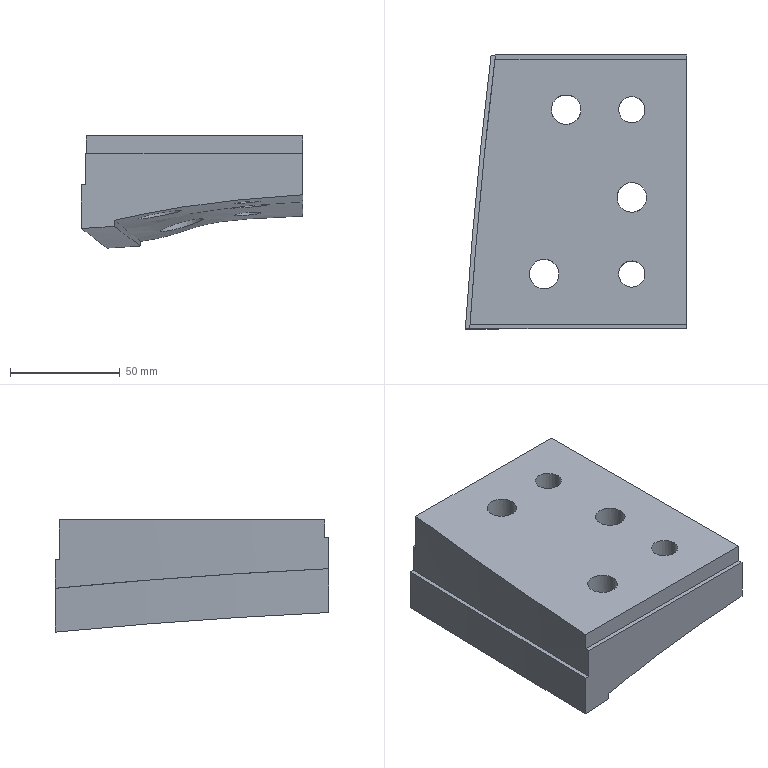Part | NX | features solid 2 | 1 solid | 25 faces | box 100.952 x 125 x 51.2 mm | volume 397040 mm3 | plane 10 | cylinder 8 | spline 7 | commonest cylinder face diameters 13.5 x3 20 x3 12 x2
STEP:
#1=CARTESIAN_POINT('',(-489.032,184.382,-45.));
#2=VERTEX_POINT('',#1);
#3=CARTESIAN_POINT('',(-490.817,179.819,-44.656));
#4=CARTESIAN_POINT('',(-488.384,184.323,-44.95));
#5=CARTESIAN_POINT('',(-489.838,189.179,-45.548));
#6=CARTESIAN_POINT('',(-494.281,191.609,-46.129));
#7=CARTESIAN_POINT('',(-499.185,190.178,-46.439));
#8=CARTESIAN_POINT('',(-501.615,185.671,-46.201));
#9=CARTESIAN_POINT('',(-500.164,180.829,-45.55));
#10=CARTESIAN_POINT('',(-495.732,178.391,-44.896));
#11=CARTESIAN_POINT('',(-490.817,179.819,-44.656));
#12=CARTESIAN_POINT('',(-488.384,184.323,-44.95));
#13=CARTESIAN_POINT('',(-489.838,189.179,-45.548));
#14=B_SPLINE_CURVE_WITH_KNOTS('',3,(#3,#4,#5,#6,#7,#8,#9,#10,#11,#12,#13),.UNSPECIFIED.,.T.,.F.,(1,1,1,1,1,1,1,1,1,1,1,1,1,1,1),(-0.01413,-0.009419,-0.00471,0.,0.00471,0.009419,0.01413,0.01884,0.02355,0.02826,0.03297,0.03768,0.04239,0.0471,0.05181),.UNSPECIFIED.);
#15=EDGE_CURVE('',#2,#2,#14,.T.);
#16=ORIENTED_EDGE('',*,*,#15,.T.);
#17=EDGE_LOOP('',(#16));
#18=FACE_BOUND('',#17,.T.);
#19=CARTESIAN_POINT('',(-485.058,146.073,-41.181));
#20=VERTEX_POINT('',#19);
#21=CARTESIAN_POINT('',(-488.05,153.62,-41.932));
#22=CARTESIAN_POINT('',(-483.979,146.199,-41.004));
#23=CARTESIAN_POINT('',(-486.381,138.023,-41.137));
#24=CARTESIAN_POINT('',(-492.586,134.671,-41.575));
#25=CARTESIAN_POINT('',(-497.883,135.157,-42.166));
#26=CARTESIAN_POINT('',(-501.42,136.996,-42.631));
#27=CARTESIAN_POINT('',(-504.,140.069,-42.843));
#28=CARTESIAN_POINT('',(-505.202,143.899,-42.744));
#29=CARTESIAN_POINT('',(-504.844,147.89,-42.805));
#30=CARTESIAN_POINT('',(-502.374,152.636,-42.99));
#31=CARTESIAN_POINT('',(-496.153,156.023,-42.778));
#32=CARTESIAN_POINT('',(-488.05,153.62,-41.932));
#33=CARTESIAN_POINT('',(-483.979,146.199,-41.004));
#34=CARTESIAN_POINT('',(-486.381,138.023,-41.137));
#35=B_SPLINE_CURVE_WITH_KNOTS('',3,(#21,#22,#23,#24,#25,#26,#27,#28,#29,#30,#31,#32,#33,#34),.UNSPECIFIED.,.T.,.F.,(1,1,1,1,1,1,1,1,1,1,1,1,1,1,1,1,1,1),(-0.0235,-0.01567,-0.007835,0.,0.007835,0.01567,0.01959,0.0235,0.02742,0.03134,0.03526,0.03917,0.04701,0.05484,0.06268,0.07051,0.07835,0.08226),.UNSPECIFIED.);
#36=EDGE_CURVE('',#20,#20,#35,.T.);
#37=ORIENTED_EDGE('',*,*,#36,.F.);
#38=EDGE_LOOP('',(#37));
#39=FACE_BOUND('',#38,.T.);
#40=CARTESIAN_POINT('',(-489.032,109.384,-39.583));
#41=VERTEX_POINT('',#40);
#42=CARTESIAN_POINT('',(-490.822,104.819,-39.486));
#43=CARTESIAN_POINT('',(-488.38,109.321,-39.523));
#44=CARTESIAN_POINT('',(-489.848,114.196,-39.92));
#45=CARTESIAN_POINT('',(-494.297,116.607,-40.474));
#46=CARTESIAN_POINT('',(-499.179,115.178,-40.9));
#47=CARTESIAN_POINT('',(-501.618,110.678,-40.908));
#48=CARTESIAN_POINT('',(-500.157,105.813,-40.46));
#49=CARTESIAN_POINT('',(-495.712,103.393,-39.862));
#50=CARTESIAN_POINT('',(-490.822,104.819,-39.486));
#51=CARTESIAN_POINT('',(-488.38,109.321,-39.523));
#52=CARTESIAN_POINT('',(-489.848,114.196,-39.92));
#53=B_SPLINE_CURVE_WITH_KNOTS('',3,(#42,#43,#44,#45,#46,#47,#48,#49,#50,#51,#52),.UNSPECIFIED.,.T.,.F.,(1,1,1,1,1,1,1,1,1,1,1,1,1,1,1),(-0.01411,-0.009409,-0.004704,0.,0.004704,0.009409,0.01411,0.01882,0.02352,0.02823,0.03293,0.03763,0.04234,0.04704,0.05175),.UNSPECIFIED.);
#54=EDGE_CURVE('',#41,#41,#53,.T.);
#55=ORIENTED_EDGE('',*,*,#54,.T.);
#56=EDGE_LOOP('',(#55));
#57=FACE_BOUND('',#56,.T.);
#58=CARTESIAN_POINT('',(-470.,85.,-36.878));
#59=VERTEX_POINT('',#58);
#60=CARTESIAN_POINT('',(-470.,210.,-46.611));
#61=VERTEX_POINT('',#60);
#62=CARTESIAN_POINT('',(-470.,85.,-36.878));
#63=CARTESIAN_POINT('',(-470.,90.22,-37.142));
#64=CARTESIAN_POINT('',(-470.,100.66,-37.689));
#65=CARTESIAN_POINT('',(-470.,113.71,-38.361));
#66=CARTESIAN_POINT('',(-470.,124.15,-38.933));
#67=CARTESIAN_POINT('',(-470.,131.966,-39.52));
#68=CARTESIAN_POINT('',(-470.,139.786,-40.056));
#69=CARTESIAN_POINT('',(-470.,150.223,-40.671));
#70=CARTESIAN_POINT('',(-470.,160.627,-41.624));
#71=CARTESIAN_POINT('',(-470.,171.035,-42.538));
#72=CARTESIAN_POINT('',(-470.,178.828,-43.35));
#73=CARTESIAN_POINT('',(-470.,186.628,-44.098));
#74=CARTESIAN_POINT('',(-470.,194.439,-44.73));
#75=CARTESIAN_POINT('',(-470.,202.242,-45.44));
#76=CARTESIAN_POINT('',(-470.,207.414,-46.217));
#77=CARTESIAN_POINT('',(-470.,210.,-46.611));
#78=B_SPLINE_CURVE_WITH_KNOTS('',3,(#62,#63,#64,#65,#66,#67,#68,#69,#70,#71,#72,#73,#74,#75,#76,#77),.UNSPECIFIED.,.F.,.F.,(4,1,1,1,1,1,1,1,1,1,1,1,1,4),(0.,0.01568,0.03136,0.0392,0.04704,0.05488,0.06272,0.07841,0.08625,0.09409,0.1019,0.1098,0.1176,0.1254),.UNSPECIFIED.);
#79=EDGE_CURVE('',#59,#61,#78,.T.);
#80=ORIENTED_EDGE('',*,*,#79,.F.);
#81=CARTESIAN_POINT('',(-555.921,85.,-48.486));
#82=VERTEX_POINT('',#81);
#83=CARTESIAN_POINT('',(-470.,85.,-36.878));
#84=CARTESIAN_POINT('',(-477.221,85.,-37.317));
#85=CARTESIAN_POINT('',(-491.647,85.,-38.355));
#86=CARTESIAN_POINT('',(-513.236,85.,-40.649));
#87=CARTESIAN_POINT('',(-531.108,85.,-43.363));
#88=CARTESIAN_POINT('',(-545.301,85.,-46.198));
#89=CARTESIAN_POINT('',(-552.373,85.,-47.779));
#90=CARTESIAN_POINT('',(-555.921,85.,-48.486));
#91=B_SPLINE_CURVE_WITH_KNOTS('',3,(#83,#84,#85,#86,#87,#88,#89,#90),.UNSPECIFIED.,.F.,.F.,(4,1,1,1,1,4),(0.,0.0217,0.04339,0.06509,0.07594,0.08679),.UNSPECIFIED.);
#92=EDGE_CURVE('',#59,#82,#91,.T.);
#93=ORIENTED_EDGE('',*,*,#92,.T.);
#94=CARTESIAN_POINT('',(-544.144,210.,-58.181));
#95=VERTEX_POINT('',#94);
#96=CARTESIAN_POINT('',(-555.921,85.,-48.486));
#97=CARTESIAN_POINT('',(-555.618,90.231,-48.778));
#98=CARTESIAN_POINT('',(-554.9,100.695,-49.199));
#99=CARTESIAN_POINT('',(-553.869,113.757,-49.868));
#100=CARTESIAN_POINT('',(-553.001,124.186,-50.711));
#101=CARTESIAN_POINT('',(-552.323,132.016,-51.197));
#102=CARTESIAN_POINT('',(-551.623,139.823,-51.95));
#103=CARTESIAN_POINT('',(-550.898,147.619,-52.805));
#104=CARTESIAN_POINT('',(-550.144,155.441,-53.298));
#105=CARTESIAN_POINT('',(-549.364,163.258,-53.831));
#106=CARTESIAN_POINT('',(-548.558,171.067,-54.429));
#107=CARTESIAN_POINT('',(-547.449,181.481,-55.148));
#108=CARTESIAN_POINT('',(-546.289,191.874,-56.065));
#109=CARTESIAN_POINT('',(-545.078,202.255,-57.078));
#110=CARTESIAN_POINT('',(-544.458,207.419,-57.811));
#111=CARTESIAN_POINT('',(-544.144,210.,-58.181));
#112=B_SPLINE_CURVE_WITH_KNOTS('',3,(#96,#97,#98,#99,#100,#101,#102,#103,#104,#105,#106,#107,#108,#109,#110,#111),.UNSPECIFIED.,.F.,.F.,(4,1,1,1,1,1,1,1,1,1,1,1,1,4),(0.,0.01574,0.03149,0.03936,0.04723,0.0551,0.06297,0.07084,0.07872,0.08659,0.09446,0.1102,0.1181,0.1259),.UNSPECIFIED.);
#113=EDGE_CURVE('',#82,#95,#112,.T.);
#114=ORIENTED_EDGE('',*,*,#113,.T.);
#115=CARTESIAN_POINT('',(-470.,210.,-46.611));
#116=CARTESIAN_POINT('',(-473.142,210.,-46.734));
#117=CARTESIAN_POINT('',(-479.425,210.,-46.986));
#118=CARTESIAN_POINT('',(-488.844,210.,-47.464));
#119=CARTESIAN_POINT('',(-498.259,210.,-48.122));
#120=CARTESIAN_POINT('',(-507.638,210.,-49.048));
#121=CARTESIAN_POINT('',(-516.834,210.,-50.901));
#122=CARTESIAN_POINT('',(-525.787,210.,-54.007));
#123=CARTESIAN_POINT('',(-534.818,210.,-56.749));
#124=CARTESIAN_POINT('',(-541.02,210.,-57.77));
#125=CARTESIAN_POINT('',(-544.144,210.,-58.181));
#126=B_SPLINE_CURVE_WITH_KNOTS('',3,(#115,#116,#117,#118,#119,#120,#121,#122,#123,#124,#125),.UNSPECIFIED.,.F.,.F.,(4,1,1,1,1,1,1,1,4),(0.01237,0.0218,0.03123,0.04067,0.0501,0.05953,0.06896,0.07839,0.08783),.UNSPECIFIED.);
#127=EDGE_CURVE('',#61,#95,#126,.T.);
#128=ORIENTED_EDGE('',*,*,#127,.F.);
#129=EDGE_LOOP('',(#80,#93,#114,#128));
#130=FACE_BOUND('',#129,.T.);
#131=CARTESIAN_POINT('',(-525.061,111.107,-44.092));
#132=VERTEX_POINT('',#131);
#133=CARTESIAN_POINT('',(-528.118,118.659,-45.091));
#134=CARTESIAN_POINT('',(-523.966,111.248,-43.923));
#135=CARTESIAN_POINT('',(-526.389,102.987,-43.772));
#136=CARTESIAN_POINT('',(-533.894,98.99,-44.809));
#137=CARTESIAN_POINT('',(-541.907,101.367,-46.521));
#138=CARTESIAN_POINT('',(-546.025,108.74,-47.878));
#139=CARTESIAN_POINT('',(-543.623,116.999,-48.006));
#140=CARTESIAN_POINT('',(-536.127,121.004,-46.796));
#141=CARTESIAN_POINT('',(-528.118,118.659,-45.091));
#142=CARTESIAN_POINT('',(-523.966,111.248,-43.923));
#143=CARTESIAN_POINT('',(-526.389,102.987,-43.772));
#144=B_SPLINE_CURVE_WITH_KNOTS('',3,(#133,#134,#135,#136,#137,#138,#139,#140,#141,#142,#143),.UNSPECIFIED.,.T.,.F.,(1,1,1,1,1,1,1,1,1,1,1,1,1,1,1),(-0.02369,-0.01579,-0.007895,0.,0.007895,0.01579,0.02369,0.03158,0.03948,0.04737,0.05527,0.06316,0.07106,0.07895,0.08685),.UNSPECIFIED.);
#145=EDGE_CURVE('',#132,#132,#144,.T.);
#146=ORIENTED_EDGE('',*,*,#145,.F.);
#147=EDGE_LOOP('',(#146));
#148=FACE_BOUND('',#147,.T.);
#149=CARTESIAN_POINT('',(-515.067,186.16,-48.081));
#150=VERTEX_POINT('',#149);
#151=CARTESIAN_POINT('',(-516.071,190.051,-48.693));
#152=CARTESIAN_POINT('',(-514.364,184.908,-47.814));
#153=CARTESIAN_POINT('',(-515.981,179.356,-47.499));
#154=CARTESIAN_POINT('',(-520.205,175.926,-48.09));
#155=CARTESIAN_POINT('',(-525.3,174.415,-49.332));
#156=CARTESIAN_POINT('',(-531.817,176.329,-51.579));
#157=CARTESIAN_POINT('',(-536.034,183.652,-53.385));
#158=CARTESIAN_POINT('',(-534.032,190.627,-53.73));
#159=CARTESIAN_POINT('',(-529.818,194.06,-53.026));
#160=CARTESIAN_POINT('',(-524.727,195.588,-51.756));
#161=CARTESIAN_POINT('',(-519.514,194.052,-49.991));
#162=CARTESIAN_POINT('',(-516.071,190.051,-48.693));
#163=CARTESIAN_POINT('',(-514.364,184.908,-47.814));
#164=CARTESIAN_POINT('',(-515.981,179.356,-47.499));
#165=B_SPLINE_CURVE_WITH_KNOTS('',3,(#151,#152,#153,#154,#155,#156,#157,#158,#159,#160,#161,#162,#163,#164),.UNSPECIFIED.,.T.,.F.,(1,1,1,1,1,1,1,1,1,1,1,1,1,1,1,1,1,1),(-0.01598,-0.00799,-0.003995,0.,0.00799,0.01198,0.01598,0.02397,0.03196,0.03995,0.04394,0.04794,0.05593,0.05992,0.06392,0.07191,0.0759,0.0799),.UNSPECIFIED.);
#166=EDGE_CURVE('',#150,#150,#165,.T.);
#167=ORIENTED_EDGE('',*,*,#166,.F.);
#168=EDGE_LOOP('',(#167));
#169=FACE_BOUND('',#168,.T.);
#170=CARTESIAN_POINT('',(-460.236,210.,-46.224));
#171=CARTESIAN_POINT('',(-460.402,208.227,-46.015));
#172=CARTESIAN_POINT('',(-460.814,203.794,-45.453));
#173=CARTESIAN_POINT('',(-461.733,195.358,-44.345));
#174=CARTESIAN_POINT('',(-462.841,184.682,-43.676));
#175=CARTESIAN_POINT('',(-463.729,174.009,-42.571));
#176=CARTESIAN_POINT('',(-464.671,164.665,-41.767));
#177=CARTESIAN_POINT('',(-465.319,155.367,-40.993));
#178=CARTESIAN_POINT('',(-465.637,145.924,-40.241));
#179=CARTESIAN_POINT('',(-466.776,135.731,-39.584));
#180=CARTESIAN_POINT('',(-467.28,126.264,-38.89));
#181=CARTESIAN_POINT('',(-467.918,115.603,-38.325));
#182=CARTESIAN_POINT('',(-468.419,106.237,-37.886));
#183=CARTESIAN_POINT('',(-468.993,95.595,-37.354));
#184=CARTESIAN_POINT('',(-469.29,88.96,-37.034));
#185=CARTESIAN_POINT('',(-469.48,85.,-36.847));
#186=CARTESIAN_POINT('',(-460.832,210.,-46.249));
#187=CARTESIAN_POINT('',(-460.999,208.227,-46.037));
#188=CARTESIAN_POINT('',(-461.414,203.794,-45.469));
#189=CARTESIAN_POINT('',(-462.332,195.358,-44.372));
#190=CARTESIAN_POINT('',(-463.441,184.682,-43.699));
#191=CARTESIAN_POINT('',(-464.331,174.009,-42.593));
#192=CARTESIAN_POINT('',(-465.273,164.665,-41.788));
#193=CARTESIAN_POINT('',(-465.922,155.367,-41.015));
#194=CARTESIAN_POINT('',(-466.245,145.924,-40.257));
#195=CARTESIAN_POINT('',(-467.376,135.731,-39.626));
#196=CARTESIAN_POINT('',(-467.882,126.264,-38.927));
#197=CARTESIAN_POINT('',(-468.521,115.603,-38.363));
#198=CARTESIAN_POINT('',(-469.022,106.237,-37.923));
#199=CARTESIAN_POINT('',(-469.597,95.595,-37.391));
#200=CARTESIAN_POINT('',(-469.894,88.96,-37.072));
#201=CARTESIAN_POINT('',(-470.084,85.,-36.883));
#202=CARTESIAN_POINT('',(-473.295,210.,-46.76));
#203=CARTESIAN_POINT('',(-473.479,208.227,-46.49));
#204=CARTESIAN_POINT('',(-473.937,203.794,-45.772));
#205=CARTESIAN_POINT('',(-474.839,195.358,-44.949));
#206=CARTESIAN_POINT('',(-475.975,184.682,-44.202));
#207=CARTESIAN_POINT('',(-476.895,174.009,-43.072));
#208=CARTESIAN_POINT('',(-477.842,164.665,-42.233));
#209=CARTESIAN_POINT('',(-478.513,155.367,-41.491));
#210=CARTESIAN_POINT('',(-478.929,145.924,-40.6));
#211=CARTESIAN_POINT('',(-479.904,135.731,-40.535));
#212=CARTESIAN_POINT('',(-480.465,126.264,-39.711));
#213=CARTESIAN_POINT('',(-481.107,115.603,-39.168));
#214=CARTESIAN_POINT('',(-481.621,106.237,-38.712));
#215=CARTESIAN_POINT('',(-482.207,95.595,-38.169));
#216=CARTESIAN_POINT('',(-482.509,88.96,-37.871));
#217=CARTESIAN_POINT('',(-482.705,85.,-37.654));
#218=CARTESIAN_POINT('',(-491.74,210.,-47.323));
#219=CARTESIAN_POINT('',(-491.958,208.227,-46.857));
#220=CARTESIAN_POINT('',(-492.499,203.794,-45.664));
#221=CARTESIAN_POINT('',(-493.223,195.358,-46.413));
#222=CARTESIAN_POINT('',(-494.458,184.682,-45.146));
#223=CARTESIAN_POINT('',(-495.396,174.009,-44.159));
#224=CARTESIAN_POINT('',(-496.354,164.665,-43.256));
#225=CARTESIAN_POINT('',(-497.049,155.367,-42.572));
#226=CARTESIAN_POINT('',(-497.612,145.924,-41.455));
#227=CARTESIAN_POINT('',(-498.346,135.731,-42.296));
#228=CARTESIAN_POINT('',(-498.993,126.264,-41.259));
#229=CARTESIAN_POINT('',(-499.642,115.603,-40.736));
#230=CARTESIAN_POINT('',(-500.178,106.237,-40.249));
#231=CARTESIAN_POINT('',(-500.78,95.595,-39.695));
#232=CARTESIAN_POINT('',(-501.087,88.96,-39.432));
#233=CARTESIAN_POINT('',(-501.293,85.,-39.169));
#234=CARTESIAN_POINT('',(-515.308,210.,-49.876));
#235=CARTESIAN_POINT('',(-515.383,208.227,-50.08));
#236=CARTESIAN_POINT('',(-515.547,203.794,-50.668));
#237=CARTESIAN_POINT('',(-516.964,195.358,-48.656));
#238=CARTESIAN_POINT('',(-518.105,184.682,-47.911));
#239=CARTESIAN_POINT('',(-519.113,174.009,-46.903));
#240=CARTESIAN_POINT('',(-520.049,164.665,-46.195));
#241=CARTESIAN_POINT('',(-520.752,155.367,-45.521));
#242=CARTESIAN_POINT('',(-521.536,145.924,-44.162));
#243=CARTESIAN_POINT('',(-521.95,135.731,-45.834));
#244=CARTESIAN_POINT('',(-522.72,126.264,-44.564));
#245=CARTESIAN_POINT('',(-523.391,115.603,-44.003));
#246=CARTESIAN_POINT('',(-523.962,106.237,-43.458));
#247=CARTESIAN_POINT('',(-524.585,95.595,-42.914));
#248=CARTESIAN_POINT('',(-524.893,88.96,-42.673));
#249=CARTESIAN_POINT('',(-525.118,85.,-42.375));
#250=CARTESIAN_POINT('',(-530.676,210.,-56.049));
#251=CARTESIAN_POINT('',(-530.891,208.227,-55.766));
#252=CARTESIAN_POINT('',(-531.432,203.794,-55.039));
#253=CARTESIAN_POINT('',(-532.529,195.358,-54.442));
#254=CARTESIAN_POINT('',(-533.734,184.682,-53.359));
#255=CARTESIAN_POINT('',(-534.746,174.009,-52.593));
#256=CARTESIAN_POINT('',(-535.674,164.665,-51.937));
#257=CARTESIAN_POINT('',(-536.473,155.367,-51.094));
#258=CARTESIAN_POINT('',(-537.062,145.924,-50.979));
#259=CARTESIAN_POINT('',(-538.426,135.731,-47.973));
#260=CARTESIAN_POINT('',(-538.988,126.264,-47.837));
#261=CARTESIAN_POINT('',(-539.746,115.603,-46.909));
#262=CARTESIAN_POINT('',(-540.322,106.237,-46.4));
#263=CARTESIAN_POINT('',(-540.959,95.595,-45.863));
#264=CARTESIAN_POINT('',(-541.28,88.96,-45.6));
#265=CARTESIAN_POINT('',(-541.504,85.,-45.321));
#266=CARTESIAN_POINT('',(-540.959,210.,-57.8));
#267=CARTESIAN_POINT('',(-541.189,208.227,-57.529));
#268=CARTESIAN_POINT('',(-541.763,203.794,-56.829));
#269=CARTESIAN_POINT('',(-542.769,195.358,-56.095));
#270=CARTESIAN_POINT('',(-543.985,184.682,-55.045));
#271=CARTESIAN_POINT('',(-545.01,174.009,-54.312));
#272=CARTESIAN_POINT('',(-545.933,164.665,-53.616));
#273=CARTESIAN_POINT('',(-546.774,155.367,-52.906));
#274=CARTESIAN_POINT('',(-547.385,145.924,-52.438));
#275=CARTESIAN_POINT('',(-548.794,135.731,-50.689));
#276=CARTESIAN_POINT('',(-549.359,126.264,-50.207));
#277=CARTESIAN_POINT('',(-550.134,115.603,-49.305));
#278=CARTESIAN_POINT('',(-550.722,106.237,-48.739));
#279=CARTESIAN_POINT('',(-551.359,95.595,-48.242));
#280=CARTESIAN_POINT('',(-551.705,88.96,-47.933));
#281=CARTESIAN_POINT('',(-551.912,85.,-47.697));
#282=CARTESIAN_POINT('',(-545.458,210.,-58.347));
#283=CARTESIAN_POINT('',(-545.688,208.227,-58.102));
#284=CARTESIAN_POINT('',(-546.261,203.794,-57.465));
#285=CARTESIAN_POINT('',(-547.264,195.358,-56.552));
#286=CARTESIAN_POINT('',(-548.481,184.682,-55.532));
#287=CARTESIAN_POINT('',(-549.517,174.009,-54.789));
#288=CARTESIAN_POINT('',(-550.439,164.665,-54.063));
#289=CARTESIAN_POINT('',(-551.292,155.367,-53.425));
#290=CARTESIAN_POINT('',(-551.937,145.924,-52.754));
#291=CARTESIAN_POINT('',(-553.279,135.731,-51.737));
#292=CARTESIAN_POINT('',(-553.867,126.264,-51.07));
#293=CARTESIAN_POINT('',(-554.644,115.603,-50.203));
#294=CARTESIAN_POINT('',(-555.239,106.237,-49.615));
#295=CARTESIAN_POINT('',(-555.877,95.595,-49.132));
#296=CARTESIAN_POINT('',(-556.23,88.96,-48.813));
#297=CARTESIAN_POINT('',(-556.433,85.,-48.587));
#298=B_SPLINE_SURFACE_WITH_KNOTS('',3,3,((#170,#171,#172,#173,#174,#175,#176,#177,#178,#179,#180,#181,#182,#183,#184,#185),(#186,#187,#188,#189,#190,#191,#192,#193,#194,#195,#196,#197,#198,#199,#200,#201),(#202,#203,#204,#205,#206,#207,#208,#209,#210,#211,#212,#213,#214,#215,#216,#217),(#218,#219,#220,#221,#222,#223,#224,#225,#226,#227,#228,#229,#230,#231,#232,#233),(#234,#235,#236,#237,#238,#239,#240,#241,#242,#243,#244,#245,#246,#247,#248,#249),(#250,#251,#252,#253,#254,#255,#256,#257,#258,#259,#260,#261,#262,#263,#264,#265),(#266,#267,#268,#269,#270,#271,#272,#273,#274,#275,#276,#277,#278,#279,#280,#281),(#282,#283,#284,#285,#286,#287,#288,#289,#290,#291,#292,#293,#294,#295,#296,#297)),.UNSPECIFIED.,.F.,.F.,.F.,(4,1,1,1,1,4),(4,1,1,1,1,1,1,1,1,1,1,1,1,4),(0.9047,0.9062,0.9375,0.9531,0.9688,0.9807),(0.5208,0.5312,0.5469,0.5703,0.5938,0.6094,0.625,0.6484,0.6641,0.6875,0.7031,0.7266,0.7422,0.7653),.UNSPECIFIED.);
#299=ADVANCED_FACE('',(#18,#39,#57,#130,#148,#169),#298,.F.);
#300=CARTESIAN_POINT('',(-470.,210.,-28.));
#301=VERTEX_POINT('',#300);
#302=CARTESIAN_POINT('',(-470.,210.,-43.841));
#303=DIRECTION('',(0.,0.,1.));
#304=VECTOR('',#303,1000.);
#305=LINE('',#302,#304);
#306=EDGE_CURVE('',#301,#61,#305,.F.);
#307=ORIENTED_EDGE('',*,*,#306,.T.);
#308=ORIENTED_EDGE('',*,*,#127,.T.);
#309=CARTESIAN_POINT('',(-544.144,210.,-60.227));
#310=VERTEX_POINT('',#309);
#311=CARTESIAN_POINT('',(-544.144,210.,-63.127));
#312=DIRECTION('',(0.,0.,1.));
#313=VECTOR('',#312,1000.);
#314=LINE('',#311,#313);
#315=EDGE_CURVE('',#310,#95,#314,.T.);
#316=ORIENTED_EDGE('',*,*,#315,.F.);
#317=CARTESIAN_POINT('',(-559.253,210.,-61.2));
#318=VERTEX_POINT('',#317);
#319=CARTESIAN_POINT('',(-559.253,210.,-61.2));
#320=CARTESIAN_POINT('',(-554.217,210.,-60.868));
#321=CARTESIAN_POINT('',(-549.18,210.,-60.544));
#322=CARTESIAN_POINT('',(-544.144,210.,-60.227));
#323=B_SPLINE_CURVE_WITH_KNOTS('',3,(#319,#320,#321,#322),.UNSPECIFIED.,.F.,.F.,(4,4),(0.01195,0.02709),.UNSPECIFIED.);
#324=EDGE_CURVE('',#318,#310,#323,.T.);
#325=ORIENTED_EDGE('',*,*,#324,.F.);
#326=CARTESIAN_POINT('',(-559.253,210.,-41.2));
#327=VERTEX_POINT('',#326);
#328=CARTESIAN_POINT('',(-559.253,210.,-55.491));
#329=DIRECTION('',(0.,0.,1.));
#330=VECTOR('',#329,1000.);
#331=LINE('',#328,#330);
#332=EDGE_CURVE('',#327,#318,#331,.F.);
#333=ORIENTED_EDGE('',*,*,#332,.F.);
#334=CARTESIAN_POINT('',(-557.238,210.,-41.223));
#335=VERTEX_POINT('',#334);
#336=CARTESIAN_POINT('',(-557.238,210.,-41.223));
#337=CARTESIAN_POINT('',(-557.91,210.,-41.215));
#338=CARTESIAN_POINT('',(-558.581,210.,-41.208));
#339=CARTESIAN_POINT('',(-559.253,210.,-41.2));
#340=B_SPLINE_CURVE_WITH_KNOTS('',3,(#336,#337,#338,#339),.UNSPECIFIED.,.F.,.F.,(4,4),(0.,0.002015),.UNSPECIFIED.);
#341=EDGE_CURVE('',#335,#327,#340,.T.);
#342=ORIENTED_EDGE('',*,*,#341,.F.);
#343=CARTESIAN_POINT('',(-557.238,210.,-28.));
#344=VERTEX_POINT('',#343);
#345=CARTESIAN_POINT('',(-557.238,210.,-8.291));
#346=DIRECTION('',(0.,0.,1.));
#347=VECTOR('',#346,1000.);
#348=LINE('',#345,#347);
#349=EDGE_CURVE('',#344,#335,#348,.F.);
#350=ORIENTED_EDGE('',*,*,#349,.F.);
#351=CARTESIAN_POINT('',(-557.238,210.,-28.));
#352=DIRECTION('',(-1.,0.,0.));
#353=VECTOR('',#352,1000.);
#354=LINE('',#351,#353);
#355=EDGE_CURVE('',#344,#301,#354,.F.);
#356=ORIENTED_EDGE('',*,*,#355,.T.);
#357=EDGE_LOOP('',(#307,#308,#316,#325,#333,#342,#350,#356));
#358=FACE_BOUND('',#357,.T.);
#359=CARTESIAN_POINT('',(-130.,210.,-36.981));
#360=DIRECTION('',(0.,1.,0.));
#361=DIRECTION('',(0.,0.,1.));
#362=AXIS2_PLACEMENT_3D('',#359,#360,#361);
#363=PLANE('',#362);
#364=ADVANCED_FACE('',(#358),#363,.T.);
#365=CARTESIAN_POINT('',(-470.,208.,-10.));
#366=VERTEX_POINT('',#365);
#367=CARTESIAN_POINT('',(-470.,208.,-28.));
#368=VERTEX_POINT('',#367);
#369=CARTESIAN_POINT('',(-470.,208.,7.));
#370=DIRECTION('',(0.,0.,-1.));
#371=VECTOR('',#370,1000.);
#372=LINE('',#369,#371);
#373=EDGE_CURVE('',#366,#368,#372,.T.);
#374=ORIENTED_EDGE('',*,*,#373,.F.);
#375=CARTESIAN_POINT('',(-470.,87.,-10.));
#376=VERTEX_POINT('',#375);
#377=CARTESIAN_POINT('',(-470.,87.,-10.));
#378=CARTESIAN_POINT('',(-470.,127.333,-10.));
#379=CARTESIAN_POINT('',(-470.,167.667,-10.));
#380=CARTESIAN_POINT('',(-470.,208.,-10.));
#381=B_SPLINE_CURVE_WITH_KNOTS('',3,(#377,#378,#379,#380),.UNSPECIFIED.,.F.,.F.,(4,4),(0.3456,0.4666),.UNSPECIFIED.);
#382=EDGE_CURVE('',#376,#366,#381,.T.);
#383=ORIENTED_EDGE('',*,*,#382,.F.);
#384=CARTESIAN_POINT('',(-470.,87.,-18.));
#385=VERTEX_POINT('',#384);
#386=CARTESIAN_POINT('',(-470.,87.,12.));
#387=DIRECTION('',(0.,0.,-1.));
#388=VECTOR('',#387,1000.);
#389=LINE('',#386,#388);
#390=EDGE_CURVE('',#376,#385,#389,.T.);
#391=ORIENTED_EDGE('',*,*,#390,.T.);
#392=CARTESIAN_POINT('',(-470.,85.,-18.));
#393=VERTEX_POINT('',#392);
#394=CARTESIAN_POINT('',(-470.,85.,-18.));
#395=DIRECTION('',(0.,1.,0.));
#396=VECTOR('',#395,1000.);
#397=LINE('',#394,#396);
#398=EDGE_CURVE('',#393,#385,#397,.T.);
#399=ORIENTED_EDGE('',*,*,#398,.F.);
#400=CARTESIAN_POINT('',(-470.,85.,0.505));
#401=DIRECTION('',(0.,0.,-1.));
#402=VECTOR('',#401,1000.);
#403=LINE('',#400,#402);
#404=EDGE_CURVE('',#59,#393,#403,.F.);
#405=ORIENTED_EDGE('',*,*,#404,.F.);
#406=ORIENTED_EDGE('',*,*,#79,.T.);
#407=ORIENTED_EDGE('',*,*,#306,.F.);
#408=CARTESIAN_POINT('',(-470.,210.,-28.));
#409=DIRECTION('',(0.,1.,0.));
#410=VECTOR('',#409,1000.);
#411=LINE('',#408,#410);
#412=EDGE_CURVE('',#301,#368,#411,.F.);
#413=ORIENTED_EDGE('',*,*,#412,.T.);
#414=EDGE_LOOP('',(#374,#383,#391,#399,#405,#406,#407,#413));
#415=FACE_BOUND('',#414,.T.);
#416=CARTESIAN_POINT('',(-470.,85.,-10.));
#417=CARTESIAN_POINT('',(-470.,210.,-10.));
#418=CARTESIAN_POINT('',(-470.,85.,-46.831));
#419=CARTESIAN_POINT('',(-470.,210.,-46.831));
#420=B_SPLINE_SURFACE_WITH_KNOTS('',1,1,((#416,#417),(#418,#419)),.PLANE_SURF.,.F.,.F.,.F.,(2,2),(2,2),(0.3333,0.5147),(0.3333,0.4906),.PIECEWISE_BEZIER_KNOTS.);
#421=ADVANCED_FACE('',(#415),#420,.T.);
#422=CARTESIAN_POINT('',(-557.479,208.,-10.));
#423=VERTEX_POINT('',#422);
#424=CARTESIAN_POINT('',(-557.479,208.,-28.));
#425=VERTEX_POINT('',#424);
#426=CARTESIAN_POINT('',(-557.479,208.,-10.5));
#427=DIRECTION('',(0.,0.,1.));
#428=VECTOR('',#427,1000.);
#429=LINE('',#426,#428);
#430=EDGE_CURVE('',#423,#425,#429,.F.);
#431=ORIENTED_EDGE('',*,*,#430,.T.);
#432=CARTESIAN_POINT('',(-557.238,210.,-28.));
#433=CARTESIAN_POINT('',(-557.319,209.333,-28.));
#434=CARTESIAN_POINT('',(-557.399,208.667,-28.));
#435=CARTESIAN_POINT('',(-557.479,208.,-28.));
#436=B_SPLINE_CURVE_WITH_KNOTS('',3,(#432,#433,#434,#435),.UNSPECIFIED.,.F.,.F.,(4,4),(0.01009,0.0121),.UNSPECIFIED.);
#437=EDGE_CURVE('',#344,#425,#436,.T.);
#438=ORIENTED_EDGE('',*,*,#437,.F.);
#439=ORIENTED_EDGE('',*,*,#349,.T.);
#440=CARTESIAN_POINT('',(-568.949,85.,-32.267));
#441=VERTEX_POINT('',#440);
#442=CARTESIAN_POINT('',(-568.949,85.,-32.267));
#443=CARTESIAN_POINT('',(-568.357,95.441,-32.764));
#444=CARTESIAN_POINT('',(-566.732,116.332,-33.863));
#445=CARTESIAN_POINT('',(-563.129,158.046,-36.589));
#446=CARTESIAN_POINT('',(-559.752,189.255,-39.214));
#447=CARTESIAN_POINT('',(-557.238,210.,-41.223));
#448=B_SPLINE_CURVE_WITH_KNOTS('',3,(#442,#443,#444,#445,#446,#447),.UNSPECIFIED.,.F.,.F.,(4,1,1,4),(0.0004228,0.1177,0.2349,0.4694),.UNSPECIFIED.);
#449=EDGE_CURVE('',#335,#441,#448,.F.);
#450=ORIENTED_EDGE('',*,*,#449,.T.);
#451=CARTESIAN_POINT('',(-568.949,85.,-18.));
#452=VERTEX_POINT('',#451);
#453=CARTESIAN_POINT('',(-568.949,85.,207.733));
#454=DIRECTION('',(0.,0.,1.));
#455=VECTOR('',#454,1000.);
#456=LINE('',#453,#455);
#457=EDGE_CURVE('',#441,#452,#456,.T.);
#458=ORIENTED_EDGE('',*,*,#457,.T.);
#459=CARTESIAN_POINT('',(-568.833,87.,-18.));
#460=VERTEX_POINT('',#459);
#461=CARTESIAN_POINT('',(-568.949,85.,-18.));
#462=CARTESIAN_POINT('',(-568.911,85.667,-18.));
#463=CARTESIAN_POINT('',(-568.872,86.333,-18.));
#464=CARTESIAN_POINT('',(-568.833,87.,-18.));
#465=B_SPLINE_CURVE_WITH_KNOTS('',3,(#461,#462,#463,#464),.UNSPECIFIED.,.F.,.F.,(4,4),(0.,0.002003),.UNSPECIFIED.);
#466=EDGE_CURVE('',#452,#460,#465,.T.);
#467=ORIENTED_EDGE('',*,*,#466,.T.);
#468=CARTESIAN_POINT('',(-568.833,87.,-10.));
#469=VERTEX_POINT('',#468);
#470=CARTESIAN_POINT('',(-568.833,87.,3.21));
#471=DIRECTION('',(0.,0.,1.));
#472=VECTOR('',#471,1000.);
#473=LINE('',#470,#472);
#474=EDGE_CURVE('',#460,#469,#473,.T.);
#475=ORIENTED_EDGE('',*,*,#474,.T.);
#476=CARTESIAN_POINT('',(-568.833,87.,-10.));
#477=CARTESIAN_POINT('',(-568.231,97.11,-10.));
#478=CARTESIAN_POINT('',(-566.649,117.303,-10.));
#479=CARTESIAN_POINT('',(-563.157,157.67,-10.));
#480=CARTESIAN_POINT('',(-559.897,187.885,-10.));
#481=CARTESIAN_POINT('',(-557.479,208.,-10.));
#482=B_SPLINE_CURVE_WITH_KNOTS('',3,(#476,#477,#478,#479,#480,#481),.UNSPECIFIED.,.F.,.F.,(4,1,1,4),(0.2522,0.2826,0.313,0.3737),.UNSPECIFIED.);
#483=EDGE_CURVE('',#469,#423,#482,.T.);
#484=ORIENTED_EDGE('',*,*,#483,.T.);
#485=EDGE_LOOP('',(#431,#438,#439,#450,#458,#467,#475,#484));
#486=FACE_BOUND('',#485,.T.);
#487=CARTESIAN_POINT('',(-557.238,210.,-41.409));
#488=CARTESIAN_POINT('',(-557.238,210.,-10.007));
#489=CARTESIAN_POINT('',(-559.75,189.253,-39.4));
#490=CARTESIAN_POINT('',(-559.75,189.253,-7.998));
#491=CARTESIAN_POINT('',(-563.13,158.047,-36.776));
#492=CARTESIAN_POINT('',(-563.13,158.047,-5.373));
#493=CARTESIAN_POINT('',(-566.732,116.331,-34.05));
#494=CARTESIAN_POINT('',(-566.732,116.331,-2.647));
#495=CARTESIAN_POINT('',(-568.356,95.444,-32.95));
#496=CARTESIAN_POINT('',(-568.356,95.444,-1.547));
#497=CARTESIAN_POINT('',(-568.949,85.,-32.453));
#498=CARTESIAN_POINT('',(-568.949,85.,-1.05));
#499=B_SPLINE_SURFACE_WITH_KNOTS('',3,1,((#487,#488),(#489,#490),(#491,#492),(#493,#494),(#495,#496),(#497,#498)),.SURF_OF_LINEAR_EXTRUSION.,.F.,.F.,.F.,(4,1,1,4),(2,2),(0.5306,0.7651,0.8823,0.9996),(0.,1.),.UNSPECIFIED.);
#500=ADVANCED_FACE('',(#486),#499,.T.);
#501=ORIENTED_EDGE('',*,*,#324,.T.);
#502=CARTESIAN_POINT('',(-555.921,85.,-51.28));
#503=VERTEX_POINT('',#502);
#504=CARTESIAN_POINT('',(-555.921,85.,-51.28));
#505=CARTESIAN_POINT('',(-555.314,95.467,-51.776));
#506=CARTESIAN_POINT('',(-553.703,116.359,-52.877));
#507=CARTESIAN_POINT('',(-550.05,158.074,-55.599));
#508=CARTESIAN_POINT('',(-546.668,189.269,-58.221));
#509=CARTESIAN_POINT('',(-544.144,210.,-60.227));
#510=B_SPLINE_CURVE_WITH_KNOTS('',3,(#504,#505,#506,#507,#508,#509),.UNSPECIFIED.,.F.,.F.,(4,1,1,4),(0.,0.03147,0.06294,0.1259),.UNSPECIFIED.);
#511=EDGE_CURVE('',#503,#310,#510,.T.);
#512=ORIENTED_EDGE('',*,*,#511,.F.);
#513=CARTESIAN_POINT('',(-570.952,85.,-52.261));
#514=VERTEX_POINT('',#513);
#515=CARTESIAN_POINT('',(-570.952,85.,-52.261));
#516=CARTESIAN_POINT('',(-565.942,85.,-51.927));
#517=CARTESIAN_POINT('',(-560.932,85.,-51.6));
#518=CARTESIAN_POINT('',(-555.921,85.,-51.28));
#519=B_SPLINE_CURVE_WITH_KNOTS('',3,(#515,#516,#517,#518),.UNSPECIFIED.,.F.,.F.,(4,4),(0.002728,0.01779),.UNSPECIFIED.);
#520=EDGE_CURVE('',#514,#503,#519,.T.);
#521=ORIENTED_EDGE('',*,*,#520,.F.);
#522=CARTESIAN_POINT('',(-559.253,210.,-61.2));
#523=CARTESIAN_POINT('',(-561.762,189.256,-59.195));
#524=CARTESIAN_POINT('',(-565.139,158.054,-56.576));
#525=CARTESIAN_POINT('',(-568.737,116.349,-53.855));
#526=CARTESIAN_POINT('',(-570.36,95.463,-52.757));
#527=CARTESIAN_POINT('',(-570.952,85.,-52.261));
#528=B_SPLINE_CURVE_WITH_KNOTS('',3,(#522,#523,#524,#525,#526,#527),.UNSPECIFIED.,.F.,.F.,(4,1,1,4),(0.4563,0.5201,0.5519,0.5838),.UNSPECIFIED.);
#529=EDGE_CURVE('',#318,#514,#528,.T.);
#530=ORIENTED_EDGE('',*,*,#529,.F.);
#531=EDGE_LOOP('',(#501,#512,#521,#530));
#532=FACE_BOUND('',#531,.T.);
#533=CARTESIAN_POINT('',(-571.045,210.966,-62.09));
#534=CARTESIAN_POINT('',(-562.025,210.892,-61.469));
#535=CARTESIAN_POINT('',(-553.004,210.82,-60.871));
#536=CARTESIAN_POINT('',(-543.983,210.752,-60.295));
#537=CARTESIAN_POINT('',(-571.062,168.639,-57.649));
#538=CARTESIAN_POINT('',(-562.042,168.565,-57.034));
#539=CARTESIAN_POINT('',(-553.022,168.495,-56.443));
#540=CARTESIAN_POINT('',(-544.,168.427,-55.874));
#541=CARTESIAN_POINT('',(-571.085,126.4,-54.364));
#542=CARTESIAN_POINT('',(-562.065,126.328,-53.754));
#543=CARTESIAN_POINT('',(-553.044,126.258,-53.168));
#544=CARTESIAN_POINT('',(-544.022,126.191,-52.604));
#545=CARTESIAN_POINT('',(-571.113,84.251,-52.234));
#546=CARTESIAN_POINT('',(-562.092,84.18,-51.628));
#547=CARTESIAN_POINT('',(-553.071,84.11,-51.047));
#548=CARTESIAN_POINT('',(-544.049,84.044,-50.487));
#549=B_SPLINE_SURFACE_WITH_KNOTS('',3,3,((#533,#534,#535,#536),(#537,#538,#539,#540),(#541,#542,#543,#544),(#545,#546,#547,#548)),.UNSPECIFIED.,.F.,.F.,.F.,(4,4),(4,4),(0.5183,0.7119),(0.104,0.137),.UNSPECIFIED.);
#550=ADVANCED_FACE('',(#532),#549,.F.);
#551=ORIENTED_EDGE('',*,*,#332,.T.);
#552=ORIENTED_EDGE('',*,*,#529,.T.);
#553=CARTESIAN_POINT('',(-570.952,85.,-32.261));
#554=VERTEX_POINT('',#553);
#555=CARTESIAN_POINT('',(-570.952,85.,-41.428));
#556=DIRECTION('',(0.,0.,1.));
#557=VECTOR('',#556,1000.);
#558=LINE('',#555,#557);
#559=EDGE_CURVE('',#554,#514,#558,.F.);
#560=ORIENTED_EDGE('',*,*,#559,.F.);
#561=CARTESIAN_POINT('',(-559.253,210.,-41.2));
#562=CARTESIAN_POINT('',(-560.507,199.631,-40.198));
#563=CARTESIAN_POINT('',(-562.287,184.062,-38.792));
#564=CARTESIAN_POINT('',(-564.187,165.849,-37.319));
#565=CARTESIAN_POINT('',(-565.088,156.758,-36.627));
#566=CARTESIAN_POINT('',(-565.594,151.525,-36.241));
#567=CARTESIAN_POINT('',(-566.31,143.971,-35.695));
#568=CARTESIAN_POINT('',(-567.359,132.403,-34.906));
#569=CARTESIAN_POINT('',(-569.095,111.652,-33.617));
#570=CARTESIAN_POINT('',(-570.344,95.748,-32.771));
#571=CARTESIAN_POINT('',(-570.952,85.,-32.261));
#572=B_SPLINE_CURVE_WITH_KNOTS('',3,(#561,#562,#563,#564,#565,#566,#567,#568,#569,#570,#571),.UNSPECIFIED.,.F.,.F.,(4,1,1,1,1,1,1,1,4),(0.5314,0.6485,0.7071,0.7364,0.7511,0.7657,0.8243,0.8828,1.),.UNSPECIFIED.);
#573=EDGE_CURVE('',#327,#554,#572,.T.);
#574=ORIENTED_EDGE('',*,*,#573,.F.);
#575=EDGE_LOOP('',(#551,#552,#560,#574));
#576=FACE_BOUND('',#575,.T.);
#577=CARTESIAN_POINT('',(-570.952,85.,-61.373));
#578=CARTESIAN_POINT('',(-570.952,85.,-32.088));
#579=CARTESIAN_POINT('',(-570.36,95.462,-61.373));
#580=CARTESIAN_POINT('',(-570.36,95.462,-32.088));
#581=CARTESIAN_POINT('',(-568.736,116.356,-61.373));
#582=CARTESIAN_POINT('',(-568.736,116.356,-32.088));
#583=CARTESIAN_POINT('',(-565.137,158.077,-61.373));
#584=CARTESIAN_POINT('',(-565.137,158.077,-32.088));
#585=CARTESIAN_POINT('',(-561.761,189.265,-61.373));
#586=CARTESIAN_POINT('',(-561.761,189.265,-32.088));
#587=CARTESIAN_POINT('',(-559.253,210.,-61.373));
#588=CARTESIAN_POINT('',(-559.253,210.,-32.088));
#589=B_SPLINE_SURFACE_WITH_KNOTS('',3,1,((#577,#578),(#579,#580),(#581,#582),(#583,#584),(#585,#586),(#587,#588)),.SURF_OF_LINEAR_EXTRUSION.,.F.,.F.,.F.,(4,1,1,4),(2,2),(0.2422,0.2639,0.2856,0.3289),(0.,1.),.UNSPECIFIED.);
#590=ADVANCED_FACE('',(#576),#589,.F.);
#591=ORIENTED_EDGE('',*,*,#341,.T.);
#592=ORIENTED_EDGE('',*,*,#573,.T.);
#593=CARTESIAN_POINT('',(-570.952,85.,-32.261));
#594=CARTESIAN_POINT('',(-570.284,85.,-32.263));
#595=CARTESIAN_POINT('',(-569.617,85.,-32.265));
#596=CARTESIAN_POINT('',(-568.949,85.,-32.267));
#597=B_SPLINE_CURVE_WITH_KNOTS('',3,(#593,#594,#595,#596),.UNSPECIFIED.,.F.,.F.,(4,4),(0.,0.002003),.UNSPECIFIED.);
#598=EDGE_CURVE('',#554,#441,#597,.T.);
#599=ORIENTED_EDGE('',*,*,#598,.T.);
#600=ORIENTED_EDGE('',*,*,#449,.F.);
#601=EDGE_LOOP('',(#591,#592,#599,#600));
#602=FACE_BOUND('',#601,.T.);
#603=CARTESIAN_POINT('',(-557.148,210.747,-41.296));
#604=CARTESIAN_POINT('',(-559.535,191.091,-39.386));
#605=CARTESIAN_POINT('',(-561.681,171.375,-37.708));
#606=CARTESIAN_POINT('',(-564.637,140.53,-35.451));
#607=CARTESIAN_POINT('',(-565.615,129.414,-34.712));
#608=CARTESIAN_POINT('',(-567.44,107.156,-33.38));
#609=CARTESIAN_POINT('',(-568.325,96.02,-32.791));
#610=CARTESIAN_POINT('',(-568.955,84.887,-32.261));
#611=CARTESIAN_POINT('',(-568.969,84.636,-32.249));
#612=CARTESIAN_POINT('',(-568.984,84.385,-32.237));
#613=CARTESIAN_POINT('',(-568.998,84.135,-32.225));
#614=CARTESIAN_POINT('',(-559.133,210.989,-41.296));
#615=CARTESIAN_POINT('',(-561.523,191.316,-39.386));
#616=CARTESIAN_POINT('',(-563.671,171.583,-37.708));
#617=CARTESIAN_POINT('',(-566.629,140.712,-35.451));
#618=CARTESIAN_POINT('',(-567.608,129.585,-34.712));
#619=CARTESIAN_POINT('',(-569.433,107.311,-33.38));
#620=CARTESIAN_POINT('',(-570.32,96.168,-32.791));
#621=CARTESIAN_POINT('',(-570.952,85.,-32.261));
#622=CARTESIAN_POINT('',(-570.966,84.748,-32.249));
#623=CARTESIAN_POINT('',(-570.981,84.497,-32.237));
#624=CARTESIAN_POINT('',(-570.995,84.245,-32.225));
#625=B_SPLINE_SURFACE_WITH_KNOTS('',1,3,((#603,#604,#605,#606,#607,#608,#609,#610,#611,#612,#613),(#614,#615,#616,#617,#618,#619,#620,#621,#622,#623,#624)),.RULED_SURF.,.F.,.F.,.F.,(2,2),(4,2,2,3,4),(0.,1.),(0.5278,0.75,0.875,1.,1.003),.UNSPECIFIED.);
#626=ADVANCED_FACE('',(#602),#625,.T.);
#627=ORIENTED_EDGE('',*,*,#315,.T.);
#628=ORIENTED_EDGE('',*,*,#113,.F.);
#629=CARTESIAN_POINT('',(-555.921,85.,-96.));
#630=DIRECTION('',(0.,0.,1.));
#631=VECTOR('',#630,1000.);
#632=LINE('',#629,#631);
#633=EDGE_CURVE('',#503,#82,#632,.T.);
#634=ORIENTED_EDGE('',*,*,#633,.F.);
#635=ORIENTED_EDGE('',*,*,#511,.T.);
#636=EDGE_LOOP('',(#627,#628,#634,#635));
#637=FACE_BOUND('',#636,.T.);
#638=CARTESIAN_POINT('',(-544.144,210.,-60.297));
#639=CARTESIAN_POINT('',(-544.144,210.,-48.415));
#640=CARTESIAN_POINT('',(-545.406,199.636,-60.297));
#641=CARTESIAN_POINT('',(-545.406,199.636,-48.415));
#642=CARTESIAN_POINT('',(-547.198,184.051,-60.297));
#643=CARTESIAN_POINT('',(-547.198,184.051,-48.415));
#644=CARTESIAN_POINT('',(-549.107,165.836,-60.297));
#645=CARTESIAN_POINT('',(-549.107,165.836,-48.415));
#646=CARTESIAN_POINT('',(-550.15,155.377,-60.297));
#647=CARTESIAN_POINT('',(-550.15,155.377,-48.415));
#648=CARTESIAN_POINT('',(-550.897,147.622,-60.297));
#649=CARTESIAN_POINT('',(-550.897,147.622,-48.415));
#650=CARTESIAN_POINT('',(-551.62,139.858,-60.297));
#651=CARTESIAN_POINT('',(-551.62,139.858,-48.415));
#652=CARTESIAN_POINT('',(-552.205,133.338,-60.297));
#653=CARTESIAN_POINT('',(-552.205,133.338,-48.415));
#654=CARTESIAN_POINT('',(-552.662,128.102,-60.297));
#655=CARTESIAN_POINT('',(-552.662,128.102,-48.415));
#656=CARTESIAN_POINT('',(-552.944,124.815,-60.297));
#657=CARTESIAN_POINT('',(-552.944,124.815,-48.415));
#658=CARTESIAN_POINT('',(-553.165,122.189,-60.297));
#659=CARTESIAN_POINT('',(-553.165,122.189,-48.415));
#660=CARTESIAN_POINT('',(-553.305,120.522,-60.297));
#661=CARTESIAN_POINT('',(-553.305,120.522,-48.415));
#662=CARTESIAN_POINT('',(-553.398,119.401,-60.297));
#663=CARTESIAN_POINT('',(-553.398,119.401,-48.415));
#664=CARTESIAN_POINT('',(-553.457,118.686,-60.297));
#665=CARTESIAN_POINT('',(-553.457,118.686,-48.415));
#666=CARTESIAN_POINT('',(-553.56,117.439,-60.297));
#667=CARTESIAN_POINT('',(-553.56,117.439,-48.415));
#668=CARTESIAN_POINT('',(-553.77,114.882,-60.297));
#669=CARTESIAN_POINT('',(-553.77,114.882,-48.415));
#670=CARTESIAN_POINT('',(-554.081,111.016,-60.297));
#671=CARTESIAN_POINT('',(-554.081,111.016,-48.415));
#672=CARTESIAN_POINT('',(-554.54,105.168,-60.297));
#673=CARTESIAN_POINT('',(-554.54,105.168,-48.415));
#674=CARTESIAN_POINT('',(-555.047,98.404,-60.297));
#675=CARTESIAN_POINT('',(-555.047,98.404,-48.415));
#676=CARTESIAN_POINT('',(-555.548,91.184,-60.297));
#677=CARTESIAN_POINT('',(-555.548,91.184,-48.415));
#678=CARTESIAN_POINT('',(-555.807,86.962,-60.297));
#679=CARTESIAN_POINT('',(-555.807,86.962,-48.415));
#680=CARTESIAN_POINT('',(-555.921,85.,-60.297));
#681=CARTESIAN_POINT('',(-555.921,85.,-48.415));
#682=B_SPLINE_SURFACE_WITH_KNOTS('',3,1,((#638,#639),(#640,#641),(#642,#643),(#644,#645),(#646,#647),(#648,#649),(#650,#651),(#652,#653),(#654,#655),(#656,#657),(#658,#659),(#660,#661),(#662,#663),(#664,#665),(#666,#667),(#668,#669),(#670,#671),(#672,#673),(#674,#675),(#676,#677),(#678,#679),(#680,#681)),.SURF_OF_LINEAR_EXTRUSION.,.F.,.F.,.F.,(4,1,1,1,1,1,1,1,1,1,1,1,1,1,1,1,1,1,1,4),(2,2),(0.5337,0.6508,0.7093,0.7386,0.7679,0.7971,0.8264,0.841,0.8557,0.863,0.8703,0.874,0.8758,0.8776,0.8849,0.8996,0.9142,0.9435,0.9727,1.002),(0.,1.),.UNSPECIFIED.);
#683=ADVANCED_FACE('',(#637),#682,.F.);
#684=CARTESIAN_POINT('',(-489.,185.,-10.));
#685=VERTEX_POINT('',#684);
#686=CARTESIAN_POINT('',(-495.,185.,-10.));
#687=DIRECTION('',(0.,0.,1.));
#688=DIRECTION('',(1.,0.,0.));
#689=AXIS2_PLACEMENT_3D('',#686,#687,#688);
#690=CIRCLE('',#689,6.);
#691=EDGE_CURVE('',#685,#685,#690,.F.);
#692=ORIENTED_EDGE('',*,*,#691,.T.);
#693=EDGE_LOOP('',(#692));
#694=FACE_BOUND('',#693,.T.);
#695=CARTESIAN_POINT('',(-531.75,185.,-10.));
#696=VERTEX_POINT('',#695);
#697=CARTESIAN_POINT('',(-525.,185.,-10.));
#698=DIRECTION('',(0.,0.,-1.));
#699=DIRECTION('',(-1.,0.,0.));
#700=AXIS2_PLACEMENT_3D('',#697,#698,#699);
#701=CIRCLE('',#700,6.75);
#702=EDGE_CURVE('',#696,#696,#701,.T.);
#703=ORIENTED_EDGE('',*,*,#702,.T.);
#704=EDGE_LOOP('',(#703));
#705=FACE_BOUND('',#704,.T.);
#706=CARTESIAN_POINT('',(-501.75,145.,-10.));
#707=VERTEX_POINT('',#706);
#708=CARTESIAN_POINT('',(-495.,145.,-10.));
#709=DIRECTION('',(0.,0.,-1.));
#710=DIRECTION('',(-1.,0.,0.));
#711=AXIS2_PLACEMENT_3D('',#708,#709,#710);
#712=CIRCLE('',#711,6.75);
#713=EDGE_CURVE('',#707,#707,#712,.T.);
#714=ORIENTED_EDGE('',*,*,#713,.T.);
#715=EDGE_LOOP('',(#714));
#716=FACE_BOUND('',#715,.T.);
#717=CARTESIAN_POINT('',(-489.,110.,-10.));
#718=VERTEX_POINT('',#717);
#719=CARTESIAN_POINT('',(-495.,110.,-10.));
#720=DIRECTION('',(0.,0.,1.));
#721=DIRECTION('',(1.,0.,0.));
#722=AXIS2_PLACEMENT_3D('',#719,#720,#721);
#723=CIRCLE('',#722,6.);
#724=EDGE_CURVE('',#718,#718,#723,.F.);
#725=ORIENTED_EDGE('',*,*,#724,.T.);
#726=EDGE_LOOP('',(#725));
#727=FACE_BOUND('',#726,.T.);
#728=CARTESIAN_POINT('',(-541.75,110.,-10.));
#729=VERTEX_POINT('',#728);
#730=CARTESIAN_POINT('',(-535.,110.,-10.));
#731=DIRECTION('',(0.,0.,-1.));
#732=DIRECTION('',(-1.,0.,0.));
#733=AXIS2_PLACEMENT_3D('',#730,#731,#732);
#734=CIRCLE('',#733,6.75);
#735=EDGE_CURVE('',#729,#729,#734,.T.);
#736=ORIENTED_EDGE('',*,*,#735,.T.);
#737=EDGE_LOOP('',(#736));
#738=FACE_BOUND('',#737,.T.);
#739=ORIENTED_EDGE('',*,*,#483,.F.);
#740=CARTESIAN_POINT('',(-470.,87.,-10.));
#741=DIRECTION('',(1.,0.,0.));
#742=VECTOR('',#741,1000.);
#743=LINE('',#740,#742);
#744=EDGE_CURVE('',#376,#469,#743,.F.);
#745=ORIENTED_EDGE('',*,*,#744,.F.);
#746=ORIENTED_EDGE('',*,*,#382,.T.);
#747=CARTESIAN_POINT('',(-557.238,208.,-10.));
#748=DIRECTION('',(-1.,0.,0.));
#749=VECTOR('',#748,1000.);
#750=LINE('',#747,#749);
#751=EDGE_CURVE('',#423,#366,#750,.F.);
#752=ORIENTED_EDGE('',*,*,#751,.F.);
#753=EDGE_LOOP('',(#739,#745,#746,#752));
#754=FACE_BOUND('',#753,.T.);
#755=CARTESIAN_POINT('',(0.,0.,-10.));
#756=DIRECTION('',(0.,0.,1.));
#757=DIRECTION('',(-1.,0.,0.));
#758=AXIS2_PLACEMENT_3D('',#755,#756,#757);
#759=PLANE('',#758);
#760=ADVANCED_FACE('',(#694,#705,#716,#727,#738,#754),#759,.T.);
#761=ORIENTED_EDGE('',*,*,#744,.T.);
#762=ORIENTED_EDGE('',*,*,#474,.F.);
#763=CARTESIAN_POINT('',(-470.,87.,-18.));
#764=DIRECTION('',(-1.,0.,0.));
#765=VECTOR('',#764,1000.);
#766=LINE('',#763,#765);
#767=EDGE_CURVE('',#385,#460,#766,.T.);
#768=ORIENTED_EDGE('',*,*,#767,.F.);
#769=ORIENTED_EDGE('',*,*,#390,.F.);
#770=EDGE_LOOP('',(#761,#762,#768,#769));
#771=FACE_BOUND('',#770,.T.);
#772=CARTESIAN_POINT('',(-470.,87.,12.));
#773=DIRECTION('',(0.,-1.,0.));
#774=DIRECTION('',(-1.,0.,0.));
#775=AXIS2_PLACEMENT_3D('',#772,#773,#774);
#776=PLANE('',#775);
#777=ADVANCED_FACE('',(#771),#776,.T.);
#778=ORIENTED_EDGE('',*,*,#404,.T.);
#779=CARTESIAN_POINT('',(-470.,85.,-18.));
#780=DIRECTION('',(-1.,0.,0.));
#781=VECTOR('',#780,1000.);
#782=LINE('',#779,#781);
#783=EDGE_CURVE('',#393,#452,#782,.T.);
#784=ORIENTED_EDGE('',*,*,#783,.T.);
#785=ORIENTED_EDGE('',*,*,#457,.F.);
#786=ORIENTED_EDGE('',*,*,#598,.F.);
#787=ORIENTED_EDGE('',*,*,#559,.T.);
#788=ORIENTED_EDGE('',*,*,#520,.T.);
#789=ORIENTED_EDGE('',*,*,#633,.T.);
#790=ORIENTED_EDGE('',*,*,#92,.F.);
#791=EDGE_LOOP('',(#778,#784,#785,#786,#787,#788,#789,#790));
#792=FACE_BOUND('',#791,.T.);
#793=CARTESIAN_POINT('',(412.414,85.,0.505));
#794=DIRECTION('',(0.,1.,0.));
#795=DIRECTION('',(0.,0.,1.));
#796=AXIS2_PLACEMENT_3D('',#793,#794,#795);
#797=PLANE('',#796);
#798=ADVANCED_FACE('',(#792),#797,.F.);
#799=ORIENTED_EDGE('',*,*,#783,.F.);
#800=ORIENTED_EDGE('',*,*,#398,.T.);
#801=ORIENTED_EDGE('',*,*,#767,.T.);
#802=ORIENTED_EDGE('',*,*,#466,.F.);
#803=EDGE_LOOP('',(#799,#800,#801,#802));
#804=FACE_BOUND('',#803,.T.);
#805=CARTESIAN_POINT('',(-470.,85.,-18.));
#806=DIRECTION('',(0.,0.,-1.));
#807=DIRECTION('',(-1.,0.,0.));
#808=AXIS2_PLACEMENT_3D('',#805,#806,#807);
#809=PLANE('',#808);
#810=ADVANCED_FACE('',(#804),#809,.F.);
#811=ORIENTED_EDGE('',*,*,#430,.F.);
#812=ORIENTED_EDGE('',*,*,#751,.T.);
#813=ORIENTED_EDGE('',*,*,#373,.T.);
#814=CARTESIAN_POINT('',(-557.238,208.,-28.));
#815=DIRECTION('',(-1.,0.,0.));
#816=VECTOR('',#815,1000.);
#817=LINE('',#814,#816);
#818=EDGE_CURVE('',#425,#368,#817,.F.);
#819=ORIENTED_EDGE('',*,*,#818,.F.);
#820=EDGE_LOOP('',(#811,#812,#813,#819));
#821=FACE_BOUND('',#820,.T.);
#822=CARTESIAN_POINT('',(-557.238,208.,7.));
#823=DIRECTION('',(0.,1.,0.));
#824=DIRECTION('',(1.,0.,0.));
#825=AXIS2_PLACEMENT_3D('',#822,#823,#824);
#826=PLANE('',#825);
#827=ADVANCED_FACE('',(#821),#826,.T.);
#828=ORIENTED_EDGE('',*,*,#818,.T.);
#829=ORIENTED_EDGE('',*,*,#412,.F.);
#830=ORIENTED_EDGE('',*,*,#355,.F.);
#831=ORIENTED_EDGE('',*,*,#437,.T.);
#832=EDGE_LOOP('',(#828,#829,#830,#831));
#833=FACE_BOUND('',#832,.T.);
#834=CARTESIAN_POINT('',(-557.238,210.,-28.));
#835=DIRECTION('',(0.,0.,1.));
#836=DIRECTION('',(-1.,0.,0.));
#837=AXIS2_PLACEMENT_3D('',#834,#835,#836);
#838=PLANE('',#837);
#839=ADVANCED_FACE('',(#833),#838,.T.);
#840=ORIENTED_EDGE('',*,*,#145,.T.);
#841=EDGE_LOOP('',(#840));
#842=FACE_BOUND('',#841,.T.);
#843=CARTESIAN_POINT('',(-535.,120.,-25.));
#844=VERTEX_POINT('',#843);
#845=CARTESIAN_POINT('',(-535.,110.,-25.));
#846=DIRECTION('',(0.,0.,1.));
#847=DIRECTION('',(0.,1.,0.));
#848=AXIS2_PLACEMENT_3D('',#845,#846,#847);
#849=CIRCLE('',#848,10.);
#850=EDGE_CURVE('',#844,#844,#849,.T.);
#851=ORIENTED_EDGE('',*,*,#850,.T.);
#852=EDGE_LOOP('',(#851));
#853=FACE_BOUND('',#852,.T.);
#854=CARTESIAN_POINT('',(-535.,110.,-135.));
#855=DIRECTION('',(0.,0.,1.));
#856=DIRECTION('',(-1.,0.,0.));
#857=AXIS2_PLACEMENT_3D('',#854,#855,#856);
#858=CYLINDRICAL_SURFACE('',#857,10.);
#859=ADVANCED_FACE('',(#842,#853),#858,.F.);
#860=CARTESIAN_POINT('',(-535.,116.75,-25.));
#861=VERTEX_POINT('',#860);
#862=CARTESIAN_POINT('',(-535.,110.,-25.));
#863=DIRECTION('',(0.,0.,1.));
#864=DIRECTION('',(0.,1.,0.));
#865=AXIS2_PLACEMENT_3D('',#862,#863,#864);
#866=CIRCLE('',#865,6.75);
#867=EDGE_CURVE('',#861,#861,#866,.T.);
#868=ORIENTED_EDGE('',*,*,#867,.T.);
#869=EDGE_LOOP('',(#868));
#870=FACE_BOUND('',#869,.T.);
#871=ORIENTED_EDGE('',*,*,#850,.F.);
#872=EDGE_LOOP('',(#871));
#873=FACE_BOUND('',#872,.T.);
#874=CARTESIAN_POINT('',(-535.,110.,-25.));
#875=DIRECTION('',(0.,0.,-1.));
#876=DIRECTION('',(0.,1.,0.));
#877=AXIS2_PLACEMENT_3D('',#874,#875,#876);
#878=PLANE('',#877);
#879=ADVANCED_FACE('',(#870,#873),#878,.T.);
#880=ORIENTED_EDGE('',*,*,#735,.F.);
#881=EDGE_LOOP('',(#880));
#882=FACE_BOUND('',#881,.T.);
#883=ORIENTED_EDGE('',*,*,#867,.F.);
#884=EDGE_LOOP('',(#883));
#885=FACE_BOUND('',#884,.T.);
#886=CARTESIAN_POINT('',(-535.,110.,-110.));
#887=DIRECTION('',(0.,0.,1.));
#888=DIRECTION('',(-1.,0.,0.));
#889=AXIS2_PLACEMENT_3D('',#886,#887,#888);
#890=CYLINDRICAL_SURFACE('',#889,6.75);
#891=ADVANCED_FACE('',(#882,#885),#890,.F.);
#892=ORIENTED_EDGE('',*,*,#54,.F.);
#893=EDGE_LOOP('',(#892));
#894=FACE_BOUND('',#893,.T.);
#895=ORIENTED_EDGE('',*,*,#724,.F.);
#896=EDGE_LOOP('',(#895));
#897=FACE_BOUND('',#896,.T.);
#898=CARTESIAN_POINT('',(-495.,110.,-210.));
#899=DIRECTION('',(0.,0.,1.));
#900=DIRECTION('',(-1.,0.,0.));
#901=AXIS2_PLACEMENT_3D('',#898,#899,#900);
#902=CYLINDRICAL_SURFACE('',#901,6.);
#903=ADVANCED_FACE('',(#894,#897),#902,.F.);
#904=ORIENTED_EDGE('',*,*,#36,.T.);
#905=EDGE_LOOP('',(#904));
#906=FACE_BOUND('',#905,.T.);
#907=CARTESIAN_POINT('',(-495.,155.,-25.));
#908=VERTEX_POINT('',#907);
#909=CARTESIAN_POINT('',(-495.,145.,-25.));
#910=DIRECTION('',(0.,0.,1.));
#911=DIRECTION('',(0.,1.,0.));
#912=AXIS2_PLACEMENT_3D('',#909,#910,#911);
#913=CIRCLE('',#912,10.);
#914=EDGE_CURVE('',#908,#908,#913,.T.);
#915=ORIENTED_EDGE('',*,*,#914,.T.);
#916=EDGE_LOOP('',(#915));
#917=FACE_BOUND('',#916,.T.);
#918=CARTESIAN_POINT('',(-495.,145.,-135.));
#919=DIRECTION('',(0.,0.,1.));
#920=DIRECTION('',(-1.,0.,0.));
#921=AXIS2_PLACEMENT_3D('',#918,#919,#920);
#922=CYLINDRICAL_SURFACE('',#921,10.);
#923=ADVANCED_FACE('',(#906,#917),#922,.F.);
#924=CARTESIAN_POINT('',(-495.,151.75,-25.));
#925=VERTEX_POINT('',#924);
#926=CARTESIAN_POINT('',(-495.,145.,-25.));
#927=DIRECTION('',(0.,0.,1.));
#928=DIRECTION('',(0.,1.,0.));
#929=AXIS2_PLACEMENT_3D('',#926,#927,#928);
#930=CIRCLE('',#929,6.75);
#931=EDGE_CURVE('',#925,#925,#930,.T.);
#932=ORIENTED_EDGE('',*,*,#931,.T.);
#933=EDGE_LOOP('',(#932));
#934=FACE_BOUND('',#933,.T.);
#935=ORIENTED_EDGE('',*,*,#914,.F.);
#936=EDGE_LOOP('',(#935));
#937=FACE_BOUND('',#936,.T.);
#938=CARTESIAN_POINT('',(-495.,145.,-25.));
#939=DIRECTION('',(0.,0.,-1.));
#940=DIRECTION('',(0.,1.,0.));
#941=AXIS2_PLACEMENT_3D('',#938,#939,#940);
#942=PLANE('',#941);
#943=ADVANCED_FACE('',(#934,#937),#942,.T.);
#944=ORIENTED_EDGE('',*,*,#713,.F.);
#945=EDGE_LOOP('',(#944));
#946=FACE_BOUND('',#945,.T.);
#947=ORIENTED_EDGE('',*,*,#931,.F.);
#948=EDGE_LOOP('',(#947));
#949=FACE_BOUND('',#948,.T.);
#950=CARTESIAN_POINT('',(-495.,145.,-110.));
#951=DIRECTION('',(0.,0.,1.));
#952=DIRECTION('',(-1.,0.,0.));
#953=AXIS2_PLACEMENT_3D('',#950,#951,#952);
#954=CYLINDRICAL_SURFACE('',#953,6.75);
#955=ADVANCED_FACE('',(#946,#949),#954,.F.);
#956=ORIENTED_EDGE('',*,*,#166,.T.);
#957=EDGE_LOOP('',(#956));
#958=FACE_BOUND('',#957,.T.);
#959=CARTESIAN_POINT('',(-525.,195.,-25.));
#960=VERTEX_POINT('',#959);
#961=CARTESIAN_POINT('',(-525.,185.,-25.));
#962=DIRECTION('',(0.,0.,1.));
#963=DIRECTION('',(0.,1.,0.));
#964=AXIS2_PLACEMENT_3D('',#961,#962,#963);
#965=CIRCLE('',#964,10.);
#966=EDGE_CURVE('',#960,#960,#965,.T.);
#967=ORIENTED_EDGE('',*,*,#966,.T.);
#968=EDGE_LOOP('',(#967));
#969=FACE_BOUND('',#968,.T.);
#970=CARTESIAN_POINT('',(-525.,185.,-135.));
#971=DIRECTION('',(0.,0.,1.));
#972=DIRECTION('',(-1.,0.,0.));
#973=AXIS2_PLACEMENT_3D('',#970,#971,#972);
#974=CYLINDRICAL_SURFACE('',#973,10.);
#975=ADVANCED_FACE('',(#958,#969),#974,.F.);
#976=CARTESIAN_POINT('',(-525.,191.75,-25.));
#977=VERTEX_POINT('',#976);
#978=CARTESIAN_POINT('',(-525.,185.,-25.));
#979=DIRECTION('',(0.,0.,1.));
#980=DIRECTION('',(0.,1.,0.));
#981=AXIS2_PLACEMENT_3D('',#978,#979,#980);
#982=CIRCLE('',#981,6.75);
#983=EDGE_CURVE('',#977,#977,#982,.T.);
#984=ORIENTED_EDGE('',*,*,#983,.T.);
#985=EDGE_LOOP('',(#984));
#986=FACE_BOUND('',#985,.T.);
#987=ORIENTED_EDGE('',*,*,#966,.F.);
#988=EDGE_LOOP('',(#987));
#989=FACE_BOUND('',#988,.T.);
#990=CARTESIAN_POINT('',(-525.,185.,-25.));
#991=DIRECTION('',(0.,0.,-1.));
#992=DIRECTION('',(0.,1.,0.));
#993=AXIS2_PLACEMENT_3D('',#990,#991,#992);
#994=PLANE('',#993);
#995=ADVANCED_FACE('',(#986,#989),#994,.T.);
#996=ORIENTED_EDGE('',*,*,#702,.F.);
#997=EDGE_LOOP('',(#996));
#998=FACE_BOUND('',#997,.T.);
#999=ORIENTED_EDGE('',*,*,#983,.F.);
#1000=EDGE_LOOP('',(#999));
#1001=FACE_BOUND('',#1000,.T.);
#1002=CARTESIAN_POINT('',(-525.,185.,-110.));
#1003=DIRECTION('',(0.,0.,1.));
#1004=DIRECTION('',(-1.,0.,0.));
#1005=AXIS2_PLACEMENT_3D('',#1002,#1003,#1004);
#1006=CYLINDRICAL_SURFACE('',#1005,6.75);
#1007=ADVANCED_FACE('',(#998,#1001),#1006,.F.);
#1008=ORIENTED_EDGE('',*,*,#15,.F.);
#1009=EDGE_LOOP('',(#1008));
#1010=FACE_BOUND('',#1009,.T.);
#1011=ORIENTED_EDGE('',*,*,#691,.F.);
#1012=EDGE_LOOP('',(#1011));
#1013=FACE_BOUND('',#1012,.T.);
#1014=CARTESIAN_POINT('',(-495.,185.,-210.));
#1015=DIRECTION('',(0.,0.,1.));
#1016=DIRECTION('',(-1.,0.,0.));
#1017=AXIS2_PLACEMENT_3D('',#1014,#1015,#1016);
#1018=CYLINDRICAL_SURFACE('',#1017,6.);
#1019=ADVANCED_FACE('',(#1010,#1013),#1018,.F.);
#1020=CLOSED_SHELL('',(#299,#364,#421,#500,#550,#590,#626,#683,#760,#777,#798,#810,#827,#839,#859,#879,#891,#903,#923,#943,#955,#975,#995,#1007,#1019));
#1021=MANIFOLD_SOLID_BREP('',#1020);
#1022=(LENGTH_UNIT()NAMED_UNIT(*)SI_UNIT(.MILLI.,.METRE.));
#1023=UNCERTAINTY_MEASURE_WITH_UNIT(LENGTH_MEASURE(0.0508),#1022,'','');
#1024=(NAMED_UNIT(*)PLANE_ANGLE_UNIT()SI_UNIT($,.RADIAN.));
#1025=(NAMED_UNIT(*)SI_UNIT($,.STERADIAN.)SOLID_ANGLE_UNIT());
#1026=(GEOMETRIC_REPRESENTATION_CONTEXT(3)GLOBAL_UNCERTAINTY_ASSIGNED_CONTEXT((#1023))GLOBAL_UNIT_ASSIGNED_CONTEXT((#1022,#1024,#1025))REPRESENTATION_CONTEXT('',''));
#1027=ADVANCED_BREP_SHAPE_REPRESENTATION('',(#1021),#1026);